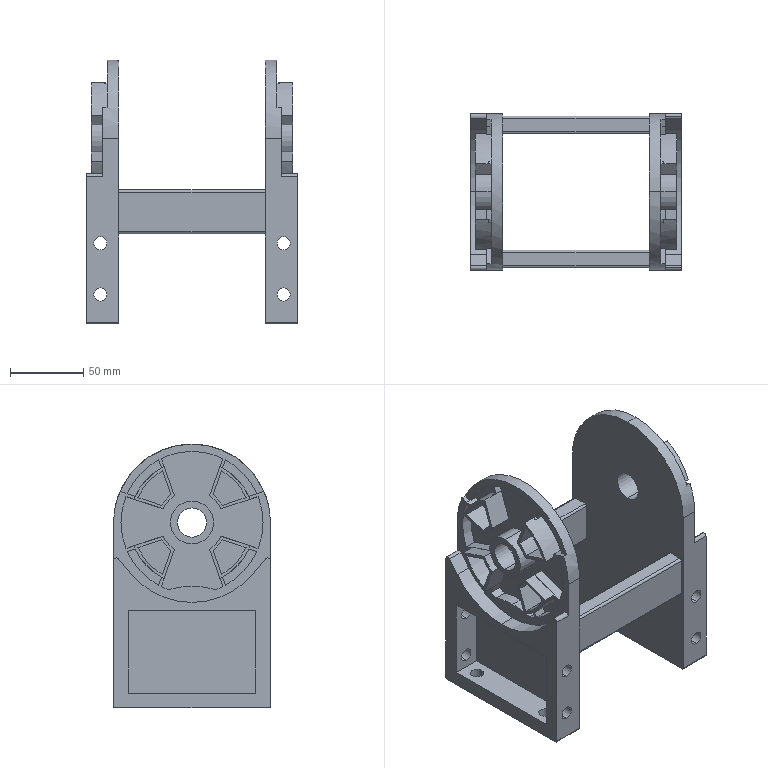Part | SolidWorks | features BaseBody 1 | 1 solid | 258 faces | box 144 x 107 x 180 mm | volume 372084 mm3 | plane 144 | cylinder 114 | commonest cylinder face diameters 9 x24 97 x19 3 x8 43.5 x8 47.5 x8 81.5 x8